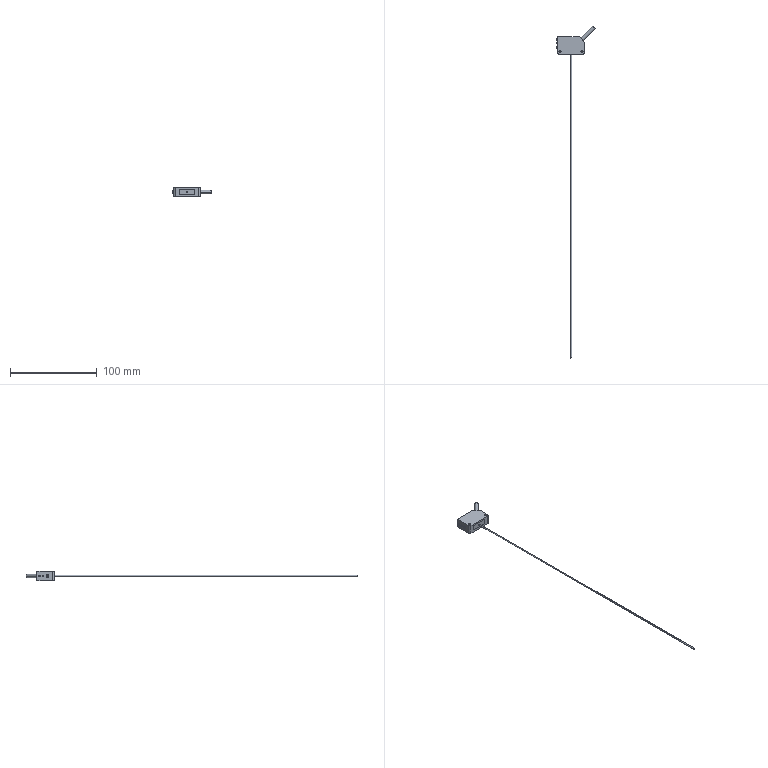Part | STEP file | 1 solid | 42 faces | box 44.556 x 382.556 x 10.8 mm | volume 7259 mm3 | cylinder 19 | plane 15 | torus 8 | commonest cylinder face diameters 2 x7 2.5 x4 4 x4 1 x2 1.5 x2